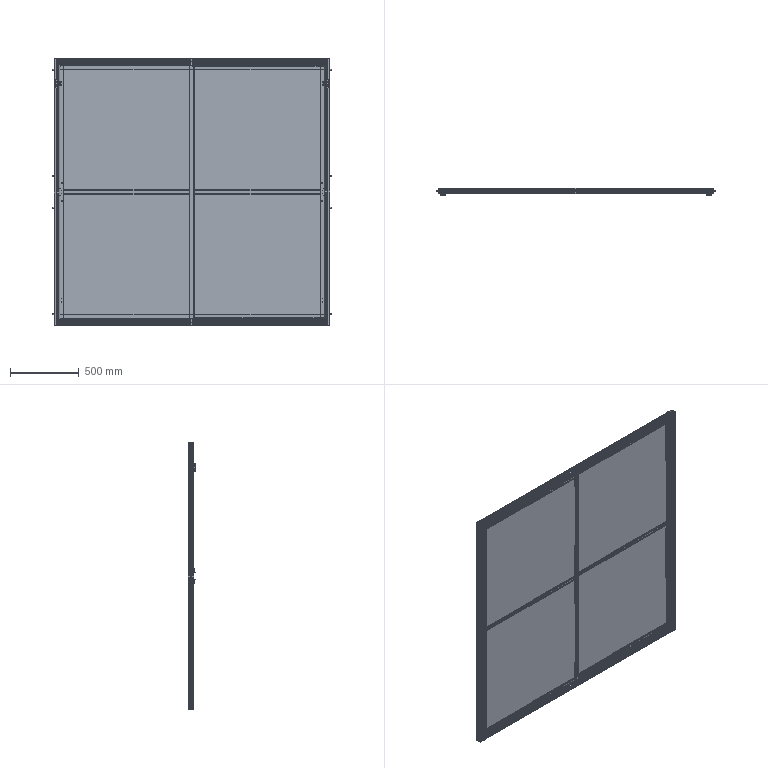Part | SolidWorks | 136 solids | 5388 faces | volume 24877160 mm3 | plane 3346 | cylinder 1374 | cone 540 | spline 128 | commonest cylinder face diameters 5 x166 11 x152 1 x112 6.8 x112 2 x100 6 x90